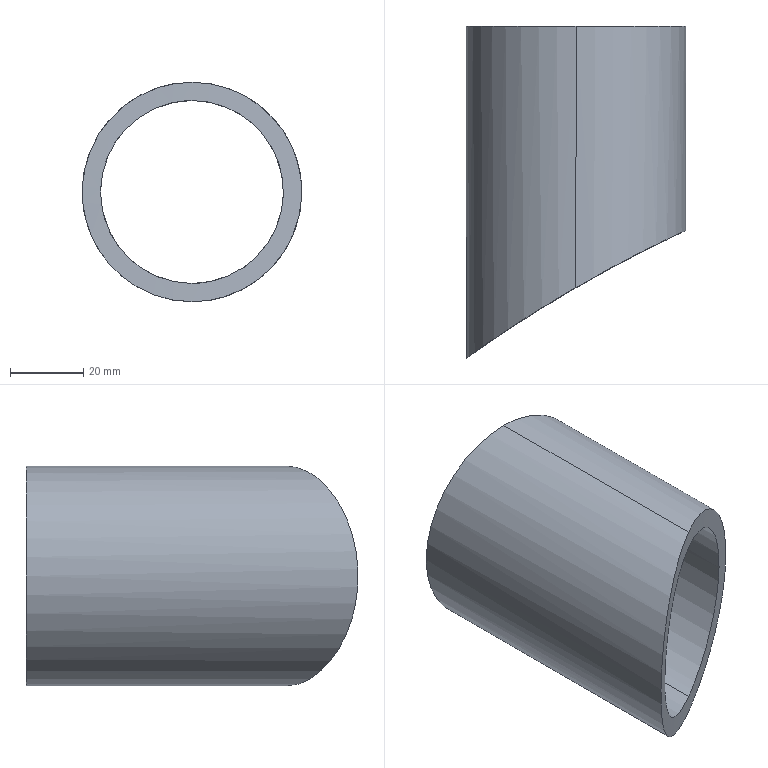Part | SolidWorks | features Extrusion 1, ICE 1 | 1 solid | 6 faces | box 60 x 90.775 x 60 mm | volume 62433 mm3 | cylinder 5 | plane 1 | commonest cylinder face diameters 50 x2 60 x2 759 x1
STEP:
#1=CARTESIAN_POINT('',(0.,400.,-25.));
#2=VERTEX_POINT('',#1);
#3=CARTESIAN_POINT('',(0.,400.,25.));
#4=VERTEX_POINT('',#3);
#5=CARTESIAN_POINT('',(0.,400.,0.));
#6=DIRECTION('',(0.,1.,0.));
#7=DIRECTION('',(0.,0.,1.));
#8=AXIS2_PLACEMENT_3D('',#5,#6,#7);
#9=CIRCLE('',#8,25.);
#10=EDGE_CURVE('',#2,#4,#9,.T.);
#11=ORIENTED_EDGE('',*,*,#10,.T.);
#12=CARTESIAN_POINT('',(0.,328.512,25.));
#13=VERTEX_POINT('',#12);
#14=CARTESIAN_POINT('',(0.,400.,25.));
#15=DIRECTION('',(0.,-1.,0.));
#16=VECTOR('',#15,1000.);
#17=LINE('',#14,#16);
#18=EDGE_CURVE('',#4,#13,#17,.T.);
#19=ORIENTED_EDGE('',*,*,#18,.T.);
#20=CARTESIAN_POINT('',(0.,328.512,-25.));
#21=VERTEX_POINT('',#20);
#22=CARTESIAN_POINT('',(0.,328.512,-25.));
#23=CARTESIAN_POINT('',(-1.557,327.612,-25.));
#24=CARTESIAN_POINT('',(-3.083,326.714,-24.856));
#25=CARTESIAN_POINT('',(-6.079,324.925,-24.297));
#26=CARTESIAN_POINT('',(-7.548,324.034,-23.883));
#27=CARTESIAN_POINT('',(-9.349,322.925,-23.189));
#28=CARTESIAN_POINT('',(-9.707,322.703,-23.042));
#29=CARTESIAN_POINT('',(-10.42,322.261,-22.728));
#30=CARTESIAN_POINT('',(-10.775,322.04,-22.562));
#31=CARTESIAN_POINT('',(-11.827,321.383,-22.04));
#32=CARTESIAN_POINT('',(-12.509,320.953,-21.659));
#33=CARTESIAN_POINT('',(-14.502,319.69,-20.424));
#34=CARTESIAN_POINT('',(-15.758,318.882,-19.474));
#35=CARTESIAN_POINT('',(-17.527,317.731,-17.845));
#36=CARTESIAN_POINT('',(-18.098,317.358,-17.267));
#37=CARTESIAN_POINT('',(-19.197,316.635,-16.037));
#38=CARTESIAN_POINT('',(-19.717,316.29,-15.393));
#39=CARTESIAN_POINT('',(-21.184,315.314,-13.38));
#40=CARTESIAN_POINT('',(-22.039,314.739,-11.928));
#41=CARTESIAN_POINT('',(-22.936,314.131,-9.955));
#42=CARTESIAN_POINT('',(-23.107,314.015,-9.553));
#43=CARTESIAN_POINT('',(-23.425,313.799,-8.743));
#44=CARTESIAN_POINT('',(-23.574,313.698,-8.335));
#45=CARTESIAN_POINT('',(-23.987,313.416,-7.097));
#46=CARTESIAN_POINT('',(-24.221,313.257,-6.256));
#47=CARTESIAN_POINT('',(-24.6,312.997,-4.542));
#48=CARTESIAN_POINT('',(-24.745,312.897,-3.67));
#49=CARTESIAN_POINT('',(-24.895,312.795,-2.335));
#50=CARTESIAN_POINT('',(-24.933,312.768,-1.884));
#51=CARTESIAN_POINT('',(-24.985,312.733,-0.9861));
#52=CARTESIAN_POINT('',(-24.998,312.724,-0.5384));
#53=CARTESIAN_POINT('',(-25.006,312.718,1.695));
#54=CARTESIAN_POINT('',(-24.824,312.844,3.462));
#55=CARTESIAN_POINT('',(-24.078,313.355,6.961));
#56=CARTESIAN_POINT('',(-23.53,313.729,8.621));
#57=CARTESIAN_POINT('',(-22.65,314.325,10.591));
#58=CARTESIAN_POINT('',(-22.464,314.451,10.98));
#59=CARTESIAN_POINT('',(-22.072,314.715,11.748));
#60=CARTESIAN_POINT('',(-21.867,314.854,12.125));
#61=CARTESIAN_POINT('',(-21.228,315.282,13.232));
#62=CARTESIAN_POINT('',(-20.772,315.588,13.937));
#63=CARTESIAN_POINT('',(-19.799,316.236,15.287));
#64=CARTESIAN_POINT('',(-19.283,316.578,15.933));
#65=CARTESIAN_POINT('',(-18.194,317.295,17.166));
#66=CARTESIAN_POINT('',(-17.619,317.671,17.755));
#67=CARTESIAN_POINT('',(-15.842,318.828,19.407));
#68=CARTESIAN_POINT('',(-14.579,319.641,20.37));
#69=CARTESIAN_POINT('',(-12.907,320.701,21.414));
#70=CARTESIAN_POINT('',(-12.568,320.915,21.615));
#71=CARTESIAN_POINT('',(-11.881,321.348,22.));
#72=CARTESIAN_POINT('',(-11.532,321.567,22.185));
#73=CARTESIAN_POINT('',(-10.481,322.224,22.711));
#74=CARTESIAN_POINT('',(-9.77,322.666,23.025));
#75=CARTESIAN_POINT('',(-7.608,323.997,23.864));
#76=CARTESIAN_POINT('',(-6.128,324.895,24.286));
#77=CARTESIAN_POINT('',(-3.85,326.256,24.714));
#78=CARTESIAN_POINT('',(-3.078,326.714,24.822));
#79=CARTESIAN_POINT('',(-1.539,327.618,24.965));
#80=CARTESIAN_POINT('',(-0.7696,328.067,25.));
#81=CARTESIAN_POINT('',(0.,328.512,25.));
#82=B_SPLINE_CURVE_WITH_KNOTS('',3,(#22,#23,#24,#25,#26,#27,#28,#29,#30,#31,#32,#33,#34,#35,#36,#37,#38,#39,#40,#41,#42,#43,#44,#45,#46,#47,#48,#49,#50,#51,#52,#53,#54,#55,#56,#57,#58,#59,#60,#61,#62,#63,#64,#65,#66,#67,#68,#69,#70,#71,#72,#73,#74,#75,#76,#77,#78,#79,#80,#81),.UNSPECIFIED.,.F.,.F.,(4,2,2,2,2,2,2,2,2,2,2,2,2,2,2,2,2,2,2,2,2,2,2,2,2,2,2,2,2,4),(0.,0.005298,0.0106,0.01192,0.01324,0.01589,0.02119,0.02384,0.02649,0.03179,0.03311,0.03443,0.03708,0.03973,0.04106,0.04238,0.04768,0.05298,0.0543,0.05563,0.05827,0.06092,0.06357,0.06887,0.07019,0.07152,0.07417,0.07947,0.08211,0.08476),.UNSPECIFIED.);
#83=EDGE_CURVE('',#21,#13,#82,.T.);
#84=ORIENTED_EDGE('',*,*,#83,.F.);
#85=CARTESIAN_POINT('',(0.,400.,-25.));
#86=DIRECTION('',(0.,-1.,0.));
#87=VECTOR('',#86,1000.);
#88=LINE('',#85,#87);
#89=EDGE_CURVE('',#2,#21,#88,.T.);
#90=ORIENTED_EDGE('',*,*,#89,.F.);
#91=EDGE_LOOP('',(#11,#19,#84,#90));
#92=FACE_OUTER_BOUND('',#91,.T.);
#93=CARTESIAN_POINT('',(0.,400.,0.));
#94=DIRECTION('',(0.,-1.,0.));
#95=DIRECTION('',(0.,0.,-1.));
#96=AXIS2_PLACEMENT_3D('',#93,#94,#95);
#97=CYLINDRICAL_SURFACE('',#96,25.);
#98=ADVANCED_FACE('',(#92),#97,.F.);
#99=CARTESIAN_POINT('',(0.,400.,30.));
#100=VERTEX_POINT('',#99);
#101=CARTESIAN_POINT('',(0.,400.,-30.));
#102=VERTEX_POINT('',#101);
#103=CARTESIAN_POINT('',(0.,400.,0.));
#104=DIRECTION('',(0.,1.,0.));
#105=DIRECTION('',(0.,0.,1.));
#106=AXIS2_PLACEMENT_3D('',#103,#104,#105);
#107=CIRCLE('',#106,30.);
#108=EDGE_CURVE('',#100,#102,#107,.T.);
#109=ORIENTED_EDGE('',*,*,#108,.F.);
#110=CARTESIAN_POINT('',(0.,328.512,30.));
#111=VERTEX_POINT('',#110);
#112=CARTESIAN_POINT('',(0.,400.,30.));
#113=DIRECTION('',(0.,-1.,0.));
#114=VECTOR('',#113,1000.);
#115=LINE('',#112,#114);
#116=EDGE_CURVE('',#100,#111,#115,.T.);
#117=ORIENTED_EDGE('',*,*,#116,.T.);
#118=CARTESIAN_POINT('',(0.,328.512,-30.));
#119=VERTEX_POINT('',#118);
#120=CARTESIAN_POINT('',(0.,328.512,30.));
#121=CARTESIAN_POINT('',(1.8,329.553,30.));
#122=CARTESIAN_POINT('',(3.604,330.577,29.839));
#123=CARTESIAN_POINT('',(5.86,331.833,29.426));
#124=CARTESIAN_POINT('',(6.311,332.083,29.332));
#125=CARTESIAN_POINT('',(7.215,332.581,29.123));
#126=CARTESIAN_POINT('',(7.666,332.829,29.008));
#127=CARTESIAN_POINT('',(9.009,333.562,28.631));
#128=CARTESIAN_POINT('',(9.89,334.038,28.338));
#129=CARTESIAN_POINT('',(12.494,335.434,27.338));
#130=CARTESIAN_POINT('',(14.177,336.318,26.508));
#131=CARTESIAN_POINT('',(16.611,337.576,24.999));
#132=CARTESIAN_POINT('',(17.41,337.985,24.451));
#133=CARTESIAN_POINT('',(18.966,338.775,23.265));
#134=CARTESIAN_POINT('',(19.714,339.151,22.635));
#135=CARTESIAN_POINT('',(21.863,340.224,20.636));
#136=CARTESIAN_POINT('',(23.172,340.867,19.16));
#137=CARTESIAN_POINT('',(24.64,341.579,17.121));
#138=CARTESIAN_POINT('',(24.925,341.717,16.703));
#139=CARTESIAN_POINT('',(25.478,341.984,15.848));
#140=CARTESIAN_POINT('',(25.746,342.112,15.408));
#141=CARTESIAN_POINT('',(26.512,342.48,14.076));
#142=CARTESIAN_POINT('',(26.976,342.701,13.165));
#143=CARTESIAN_POINT('',(28.227,343.294,10.364));
#144=CARTESIAN_POINT('',(28.875,343.597,8.406));
#145=CARTESIAN_POINT('',(29.431,343.857,5.837));
#146=CARTESIAN_POINT('',(29.529,343.903,5.319));
#147=CARTESIAN_POINT('',(29.697,343.982,4.284));
#148=CARTESIAN_POINT('',(29.767,344.014,3.765));
#149=CARTESIAN_POINT('',(29.937,344.093,2.208));
#150=CARTESIAN_POINT('',(29.995,344.12,1.167));
#151=CARTESIAN_POINT('',(30.004,344.124,-0.9204));
#152=CARTESIAN_POINT('',(29.954,344.101,-1.967));
#153=CARTESIAN_POINT('',(29.795,344.027,-3.541));
#154=CARTESIAN_POINT('',(29.728,343.996,-4.066));
#155=CARTESIAN_POINT('',(29.567,343.921,-5.104));
#156=CARTESIAN_POINT('',(29.474,343.877,-5.618));
#157=CARTESIAN_POINT('',(28.942,343.629,-8.169));
#158=CARTESIAN_POINT('',(28.311,343.333,-10.14));
#159=CARTESIAN_POINT('',(27.268,342.839,-12.518));
#160=CARTESIAN_POINT('',(27.048,342.735,-12.987));
#161=CARTESIAN_POINT('',(26.587,342.515,-13.907));
#162=CARTESIAN_POINT('',(26.346,342.4,-14.358));
#163=CARTESIAN_POINT('',(25.592,342.039,-15.687));
#164=CARTESIAN_POINT('',(25.048,341.777,-16.541));
#165=CARTESIAN_POINT('',(23.882,341.212,-18.184));
#166=CARTESIAN_POINT('',(23.26,340.908,-18.973));
#167=CARTESIAN_POINT('',(21.937,340.258,-20.489));
#168=CARTESIAN_POINT('',(21.245,339.915,-21.205));
#169=CARTESIAN_POINT('',(19.092,338.841,-23.224));
#170=CARTESIAN_POINT('',(17.553,338.061,-24.406));
#171=CARTESIAN_POINT('',(15.506,337.005,-25.687));
#172=CARTESIAN_POINT('',(15.09,336.789,-25.933));
#173=CARTESIAN_POINT('',(14.254,336.354,-26.402));
#174=CARTESIAN_POINT('',(13.832,336.133,-26.625));
#175=CARTESIAN_POINT('',(12.56,335.464,-27.261));
#176=CARTESIAN_POINT('',(11.7,335.008,-27.64));
#177=CARTESIAN_POINT('',(9.956,334.074,-28.315));
#178=CARTESIAN_POINT('',(9.074,333.597,-28.61));
#179=CARTESIAN_POINT('',(7.286,332.621,-29.116));
#180=CARTESIAN_POINT('',(6.379,332.121,-29.329));
#181=CARTESIAN_POINT('',(4.561,331.11,-29.666));
#182=CARTESIAN_POINT('',(3.65,330.598,-29.791));
#183=CARTESIAN_POINT('',(2.283,329.822,-29.917));
#184=CARTESIAN_POINT('',(1.827,329.562,-29.948));
#185=CARTESIAN_POINT('',(0.9139,329.039,-29.99));
#186=CARTESIAN_POINT('',(0.4555,328.776,-30.));
#187=CARTESIAN_POINT('',(0.,328.512,-30.));
#188=B_SPLINE_CURVE_WITH_KNOTS('',3,(#120,#121,#122,#123,#124,#125,#126,#127,#128,#129,#130,#131,#132,#133,#134,#135,#136,#137,#138,#139,#140,#141,#142,#143,#144,#145,#146,#147,#148,#149,#150,#151,#152,#153,#154,#155,#156,#157,#158,#159,#160,#161,#162,#163,#164,#165,#166,#167,#168,#169,#170,#171,#172,#173,#174,#175,#176,#177,#178,#179,#180,#181,#182,#183,#184,#185,#186,#187),.UNSPECIFIED.,.F.,.F.,(4,2,2,2,2,2,2,2,2,2,2,2,2,2,2,2,2,2,2,2,2,2,2,2,2,2,2,2,2,2,2,2,2,4),(0.102,0.1082,0.1097,0.1113,0.1144,0.1206,0.1237,0.1268,0.133,0.1345,0.1361,0.1392,0.1454,0.1469,0.1485,0.1516,0.1547,0.1562,0.1578,0.164,0.1655,0.1671,0.1702,0.1733,0.1764,0.1826,0.1841,0.1857,0.1888,0.1919,0.195,0.1981,0.1996,0.2012),.UNSPECIFIED.);
#189=EDGE_CURVE('',#111,#119,#188,.T.);
#190=ORIENTED_EDGE('',*,*,#189,.T.);
#191=CARTESIAN_POINT('',(0.,400.,-30.));
#192=DIRECTION('',(0.,-1.,0.));
#193=VECTOR('',#192,1000.);
#194=LINE('',#191,#193);
#195=EDGE_CURVE('',#102,#119,#194,.T.);
#196=ORIENTED_EDGE('',*,*,#195,.F.);
#197=EDGE_LOOP('',(#109,#117,#190,#196));
#198=FACE_OUTER_BOUND('',#197,.T.);
#199=CARTESIAN_POINT('',(0.,400.,0.));
#200=DIRECTION('',(0.,-1.,0.));
#201=DIRECTION('',(0.,0.,-1.));
#202=AXIS2_PLACEMENT_3D('',#199,#200,#201);
#203=CYLINDRICAL_SURFACE('',#202,30.);
#204=ADVANCED_FACE('',(#198),#203,.T.);
#205=CARTESIAN_POINT('',(0.,400.,0.));
#206=DIRECTION('',(0.,1.,0.));
#207=DIRECTION('',(0.,0.,1.));
#208=AXIS2_PLACEMENT_3D('',#205,#206,#207);
#209=CIRCLE('',#208,30.);
#210=EDGE_CURVE('',#102,#100,#209,.T.);
#211=ORIENTED_EDGE('',*,*,#210,.T.);
#212=ORIENTED_EDGE('',*,*,#108,.T.);
#213=EDGE_LOOP('',(#211,#212));
#214=FACE_OUTER_BOUND('',#213,.T.);
#215=ORIENTED_EDGE('',*,*,#10,.F.);
#216=CARTESIAN_POINT('',(0.,400.,0.));
#217=DIRECTION('',(0.,1.,0.));
#218=DIRECTION('',(0.,0.,1.));
#219=AXIS2_PLACEMENT_3D('',#216,#217,#218);
#220=CIRCLE('',#219,25.);
#221=EDGE_CURVE('',#4,#2,#220,.T.);
#222=ORIENTED_EDGE('',*,*,#221,.F.);
#223=EDGE_LOOP('',(#215,#222));
#224=FACE_BOUND('',#223,.T.);
#225=CARTESIAN_POINT('',(0.,400.,0.));
#226=DIRECTION('',(0.,1.,0.));
#227=DIRECTION('',(0.,0.,1.));
#228=AXIS2_PLACEMENT_3D('',#225,#226,#227);
#229=PLANE('',#228);
#230=ADVANCED_FACE('',(#214,#224),#229,.T.);
#231=ORIENTED_EDGE('',*,*,#116,.F.);
#232=ORIENTED_EDGE('',*,*,#210,.F.);
#233=ORIENTED_EDGE('',*,*,#195,.T.);
#234=CARTESIAN_POINT('',(0.,328.512,-30.));
#235=CARTESIAN_POINT('',(-1.873,327.429,-30.));
#236=CARTESIAN_POINT('',(-3.708,326.346,-29.826));
#237=CARTESIAN_POINT('',(-7.306,324.183,-29.154));
#238=CARTESIAN_POINT('',(-9.069,323.103,-28.656));
#239=CARTESIAN_POINT('',(-11.229,321.757,-27.823));
#240=CARTESIAN_POINT('',(-11.658,321.488,-27.646));
#241=CARTESIAN_POINT('',(-12.513,320.95,-27.27));
#242=CARTESIAN_POINT('',(-12.939,320.681,-27.07));
#243=CARTESIAN_POINT('',(-14.199,319.881,-26.444));
#244=CARTESIAN_POINT('',(-15.016,319.358,-25.988));
#245=CARTESIAN_POINT('',(-17.404,317.817,-24.507));
#246=CARTESIAN_POINT('',(-18.908,316.829,-23.37));
#247=CARTESIAN_POINT('',(-21.028,315.418,-21.419));
#248=CARTESIAN_POINT('',(-21.711,314.959,-20.727));
#249=CARTESIAN_POINT('',(-23.028,314.07,-19.253));
#250=CARTESIAN_POINT('',(-23.652,313.646,-18.482));
#251=CARTESIAN_POINT('',(-25.41,312.443,-16.071));
#252=CARTESIAN_POINT('',(-26.438,311.731,-14.331));
#253=CARTESIAN_POINT('',(-27.516,310.978,-11.964));
#254=CARTESIAN_POINT('',(-27.721,310.834,-11.481));
#255=CARTESIAN_POINT('',(-28.104,310.566,-10.51));
#256=CARTESIAN_POINT('',(-28.282,310.44,-10.019));
#257=CARTESIAN_POINT('',(-28.78,310.09,-8.533));
#258=CARTESIAN_POINT('',(-29.06,309.892,-7.524));
#259=CARTESIAN_POINT('',(-29.517,309.568,-5.465));
#260=CARTESIAN_POINT('',(-29.693,309.444,-4.415));
#261=CARTESIAN_POINT('',(-29.873,309.316,-2.81));
#262=CARTESIAN_POINT('',(-29.919,309.283,-2.267));
#263=CARTESIAN_POINT('',(-29.981,309.238,-1.187));
#264=CARTESIAN_POINT('',(-29.998,309.227,-0.6487));
#265=CARTESIAN_POINT('',(-30.008,309.22,2.037));
#266=CARTESIAN_POINT('',(-29.787,309.377,4.164));
#267=CARTESIAN_POINT('',(-28.888,310.014,8.372));
#268=CARTESIAN_POINT('',(-28.229,310.479,10.363));
#269=CARTESIAN_POINT('',(-26.959,311.367,13.202));
#270=CARTESIAN_POINT('',(-26.485,311.697,14.127));
#271=CARTESIAN_POINT('',(-25.464,312.403,15.894));
#272=CARTESIAN_POINT('',(-24.916,312.781,16.739));
#273=CARTESIAN_POINT('',(-23.749,313.58,18.357));
#274=CARTESIAN_POINT('',(-23.13,314.001,19.131));
#275=CARTESIAN_POINT('',(-22.15,314.663,20.239));
#276=CARTESIAN_POINT('',(-21.814,314.889,20.601));
#277=CARTESIAN_POINT('',(-21.129,315.349,21.302));
#278=CARTESIAN_POINT('',(-20.781,315.582,21.643));
#279=CARTESIAN_POINT('',(-19.008,316.763,23.291));
#280=CARTESIAN_POINT('',(-17.495,317.758,24.444));
#281=CARTESIAN_POINT('',(-15.09,319.311,25.946));
#282=CARTESIAN_POINT('',(-14.262,319.841,26.41));
#283=CARTESIAN_POINT('',(-12.583,320.907,27.25));
#284=CARTESIAN_POINT('',(-11.732,321.443,27.627));
#285=CARTESIAN_POINT('',(-9.14,323.06,28.634));
#286=CARTESIAN_POINT('',(-7.364,324.148,29.141));
#287=CARTESIAN_POINT('',(-4.626,325.795,29.656));
#288=CARTESIAN_POINT('',(-3.699,326.347,29.786));
#289=CARTESIAN_POINT('',(-1.85,327.437,29.957));
#290=CARTESIAN_POINT('',(-0.9255,327.977,30.));
#291=CARTESIAN_POINT('',(0.,328.512,30.));
#292=B_SPLINE_CURVE_WITH_KNOTS('',3,(#234,#235,#236,#237,#238,#239,#240,#241,#242,#243,#244,#245,#246,#247,#248,#249,#250,#251,#252,#253,#254,#255,#256,#257,#258,#259,#260,#261,#262,#263,#264,#265,#266,#267,#268,#269,#270,#271,#272,#273,#274,#275,#276,#277,#278,#279,#280,#281,#282,#283,#284,#285,#286,#287,#288,#289,#290,#291),.UNSPECIFIED.,.F.,.F.,(4,2,2,2,2,2,2,2,2,2,2,2,2,2,2,2,2,2,2,2,2,2,2,2,2,2,2,2,4),(0.,0.006374,0.01275,0.01434,0.01594,0.01912,0.0255,0.02868,0.03187,0.03824,0.03984,0.04143,0.04462,0.04781,0.0494,0.05099,0.05737,0.06374,0.06693,0.07011,0.0733,0.0749,0.07649,0.08286,0.08605,0.08924,0.09561,0.0988,0.102),.UNSPECIFIED.);
#293=EDGE_CURVE('',#119,#111,#292,.T.);
#294=ORIENTED_EDGE('',*,*,#293,.T.);
#295=EDGE_LOOP('',(#231,#232,#233,#294));
#296=FACE_OUTER_BOUND('',#295,.T.);
#297=CARTESIAN_POINT('',(0.,400.,0.));
#298=DIRECTION('',(0.,-1.,0.));
#299=DIRECTION('',(0.,0.,-1.));
#300=AXIS2_PLACEMENT_3D('',#297,#298,#299);
#301=CYLINDRICAL_SURFACE('',#300,30.);
#302=ADVANCED_FACE('',(#296),#301,.T.);
#303=ORIENTED_EDGE('',*,*,#18,.F.);
#304=ORIENTED_EDGE('',*,*,#221,.T.);
#305=ORIENTED_EDGE('',*,*,#89,.T.);
#306=CARTESIAN_POINT('',(0.,328.512,25.));
#307=CARTESIAN_POINT('',(1.504,329.382,25.));
#308=CARTESIAN_POINT('',(3.008,330.238,24.865));
#309=CARTESIAN_POINT('',(4.888,331.291,24.521));
#310=CARTESIAN_POINT('',(5.264,331.501,24.443));
#311=CARTESIAN_POINT('',(6.016,331.919,24.268));
#312=CARTESIAN_POINT('',(6.392,332.128,24.172));
#313=CARTESIAN_POINT('',(7.511,332.744,23.858));
#314=CARTESIAN_POINT('',(8.246,333.146,23.614));
#315=CARTESIAN_POINT('',(10.415,334.323,22.78));
#316=CARTESIAN_POINT('',(11.815,335.071,22.089));
#317=CARTESIAN_POINT('',(13.841,336.138,20.834));
#318=CARTESIAN_POINT('',(14.503,336.484,20.379));
#319=CARTESIAN_POINT('',(15.8,337.157,19.391));
#320=CARTESIAN_POINT('',(16.422,337.478,18.867));
#321=CARTESIAN_POINT('',(18.212,338.395,17.204));
#322=CARTESIAN_POINT('',(19.302,338.945,15.975));
#323=CARTESIAN_POINT('',(20.525,339.556,14.279));
#324=CARTESIAN_POINT('',(20.762,339.675,13.932));
#325=CARTESIAN_POINT('',(21.222,339.904,13.221));
#326=CARTESIAN_POINT('',(21.446,340.014,12.855));
#327=CARTESIAN_POINT('',(22.086,340.331,11.744));
#328=CARTESIAN_POINT('',(22.474,340.522,10.985));
#329=CARTESIAN_POINT('',(23.518,341.035,8.649));
#330=CARTESIAN_POINT('',(24.059,341.297,7.017));
#331=CARTESIAN_POINT('',(24.524,341.523,4.877));
#332=CARTESIAN_POINT('',(24.606,341.563,4.444));
#333=CARTESIAN_POINT('',(24.746,341.631,3.579));
#334=CARTESIAN_POINT('',(24.805,341.659,3.146));
#335=CARTESIAN_POINT('',(24.947,341.728,1.845));
#336=CARTESIAN_POINT('',(24.996,341.751,0.9758));
#337=CARTESIAN_POINT('',(25.003,341.755,-0.7664));
#338=CARTESIAN_POINT('',(24.962,341.735,-1.639));
#339=CARTESIAN_POINT('',(24.829,341.671,-2.952));
#340=CARTESIAN_POINT('',(24.773,341.643,-3.391));
#341=CARTESIAN_POINT('',(24.639,341.579,-4.258));
#342=CARTESIAN_POINT('',(24.56,341.541,-4.687));
#343=CARTESIAN_POINT('',(24.116,341.325,-6.817));
#344=CARTESIAN_POINT('',(23.588,341.069,-8.461));
#345=CARTESIAN_POINT('',(22.719,340.643,-10.442));
#346=CARTESIAN_POINT('',(22.535,340.552,-10.834));
#347=CARTESIAN_POINT('',(22.15,340.363,-11.6));
#348=CARTESIAN_POINT('',(21.949,340.263,-11.976));
#349=CARTESIAN_POINT('',(21.32,339.952,-13.084));
#350=CARTESIAN_POINT('',(20.866,339.727,-13.795));
#351=CARTESIAN_POINT('',(19.894,339.241,-15.163));
#352=CARTESIAN_POINT('',(19.376,338.981,-15.82));
#353=CARTESIAN_POINT('',(18.274,338.424,-17.081));
#354=CARTESIAN_POINT('',(17.697,338.131,-17.677));
#355=CARTESIAN_POINT('',(15.905,337.214,-19.357));
#356=CARTESIAN_POINT('',(14.624,336.55,-20.34));
#357=CARTESIAN_POINT('',(12.921,335.653,-21.406));
#358=CARTESIAN_POINT('',(12.574,335.471,-21.611));
#359=CARTESIAN_POINT('',(11.878,335.102,-22.001));
#360=CARTESIAN_POINT('',(11.528,334.915,-22.187));
#361=CARTESIAN_POINT('',(10.468,334.349,-22.716));
#362=CARTESIAN_POINT('',(9.752,333.963,-23.033));
#363=CARTESIAN_POINT('',(8.301,333.176,-23.595));
#364=CARTESIAN_POINT('',(7.566,332.774,-23.84));
#365=CARTESIAN_POINT('',(6.077,331.954,-24.262));
#366=CARTESIAN_POINT('',(5.321,331.534,-24.439));
#367=CARTESIAN_POINT('',(3.806,330.685,-24.721));
#368=CARTESIAN_POINT('',(3.046,330.256,-24.825));
#369=CARTESIAN_POINT('',(1.905,329.607,-24.93));
#370=CARTESIAN_POINT('',(1.525,329.39,-24.956));
#371=CARTESIAN_POINT('',(0.7629,328.952,-24.991));
#372=CARTESIAN_POINT('',(0.3803,328.732,-25.));
#373=CARTESIAN_POINT('',(0.,328.512,-25.));
#374=B_SPLINE_CURVE_WITH_KNOTS('',3,(#306,#307,#308,#309,#310,#311,#312,#313,#314,#315,#316,#317,#318,#319,#320,#321,#322,#323,#324,#325,#326,#327,#328,#329,#330,#331,#332,#333,#334,#335,#336,#337,#338,#339,#340,#341,#342,#343,#344,#345,#346,#347,#348,#349,#350,#351,#352,#353,#354,#355,#356,#357,#358,#359,#360,#361,#362,#363,#364,#365,#366,#367,#368,#369,#370,#371,#372,#373),.UNSPECIFIED.,.F.,.F.,(4,2,2,2,2,2,2,2,2,2,2,2,2,2,2,2,2,2,2,2,2,2,2,2,2,2,2,2,2,2,2,2,2,4),(0.08476,0.08994,0.09123,0.09253,0.09511,0.1003,0.1029,0.1055,0.1106,0.1119,0.1132,0.1158,0.121,0.1223,0.1236,0.1262,0.1288,0.13,0.1313,0.1365,0.1378,0.1391,0.1417,0.1443,0.1469,0.152,0.1533,0.1546,0.1572,0.1598,0.1624,0.165,0.1663,0.1676),.UNSPECIFIED.);
#375=EDGE_CURVE('',#13,#21,#374,.T.);
#376=ORIENTED_EDGE('',*,*,#375,.F.);
#377=EDGE_LOOP('',(#303,#304,#305,#376));
#378=FACE_OUTER_BOUND('',#377,.T.);
#379=CARTESIAN_POINT('',(0.,400.,0.));
#380=DIRECTION('',(0.,-1.,0.));
#381=DIRECTION('',(0.,0.,-1.));
#382=AXIS2_PLACEMENT_3D('',#379,#380,#381);
#383=CYLINDRICAL_SURFACE('',#382,25.);
#384=ADVANCED_FACE('',(#378),#383,.F.);
#385=ORIENTED_EDGE('',*,*,#83,.T.);
#386=ORIENTED_EDGE('',*,*,#375,.T.);
#387=EDGE_LOOP('',(#385,#386));
#388=FACE_BOUND('',#387,.T.);
#389=ORIENTED_EDGE('',*,*,#293,.F.);
#390=ORIENTED_EDGE('',*,*,#189,.F.);
#391=EDGE_LOOP('',(#389,#390));
#392=FACE_OUTER_BOUND('',#391,.T.);
#393=CARTESIAN_POINT('',(190.,0.,-30.));
#394=DIRECTION('',(0.,0.,1.));
#395=DIRECTION('',(1.,0.,0.));
#396=AXIS2_PLACEMENT_3D('',#393,#394,#395);
#397=CYLINDRICAL_SURFACE('',#396,379.5);
#398=ADVANCED_FACE('',(#388,#392),#397,.F.);
#399=CLOSED_SHELL('',(#98,#204,#230,#302,#384,#398));
#400=MANIFOLD_SOLID_BREP('',#399);
#401=CARTESIAN_POINT('',(0.,0.,0.));
#402=DIRECTION('',(0.,0.,1.));
#403=DIRECTION('',(1.,0.,0.));
#404=AXIS2_PLACEMENT_3D('',#401,#402,#403);
#405=(LENGTH_UNIT()NAMED_UNIT(*)SI_UNIT(.MILLI.,.METRE.));
#406=UNCERTAINTY_MEASURE_WITH_UNIT(LENGTH_MEASURE(0.00001),#405,'','');
#407=(NAMED_UNIT(*)PLANE_ANGLE_UNIT()SI_UNIT($,.RADIAN.));
#408=(NAMED_UNIT(*)SI_UNIT($,.STERADIAN.)SOLID_ANGLE_UNIT());
#409=(GEOMETRIC_REPRESENTATION_CONTEXT(3)GLOBAL_UNCERTAINTY_ASSIGNED_CONTEXT((#406))GLOBAL_UNIT_ASSIGNED_CONTEXT((#405,#407,#408))REPRESENTATION_CONTEXT('',''));
#410=ADVANCED_BREP_SHAPE_REPRESENTATION('',(#400,#404),#409);